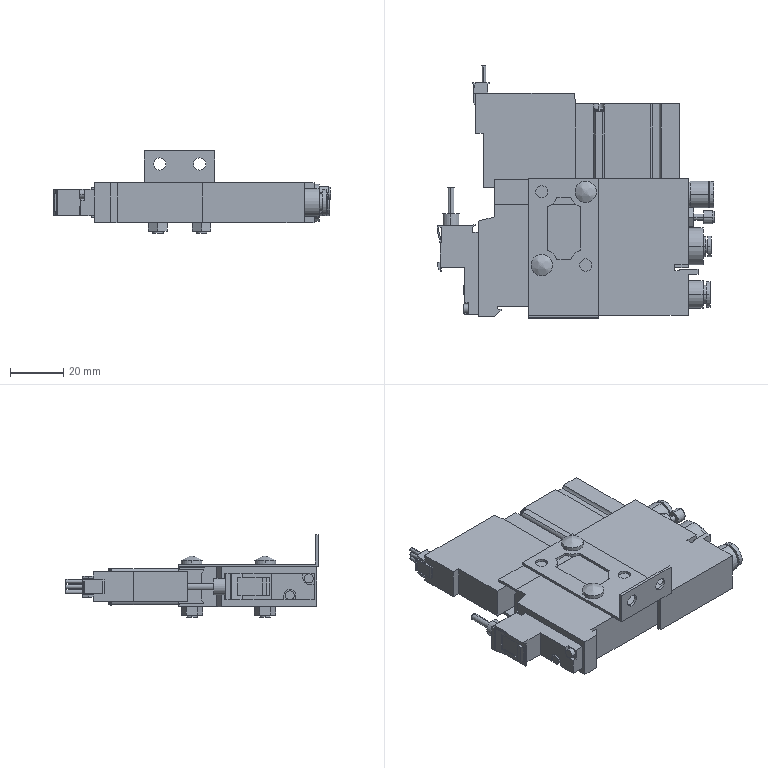Part | SolidWorks | features BaseBody 3 | 3 solids | 327 faces | box 104.2 x 94.7 x 31 mm | volume 87766 mm3 | plane 203 | cylinder 109 | cone 8 | spline 7 | commonest cylinder face diameters 4 x13 4.5 x10 4.6 x8 1.5 x6 2.5 x4 3.2 x4